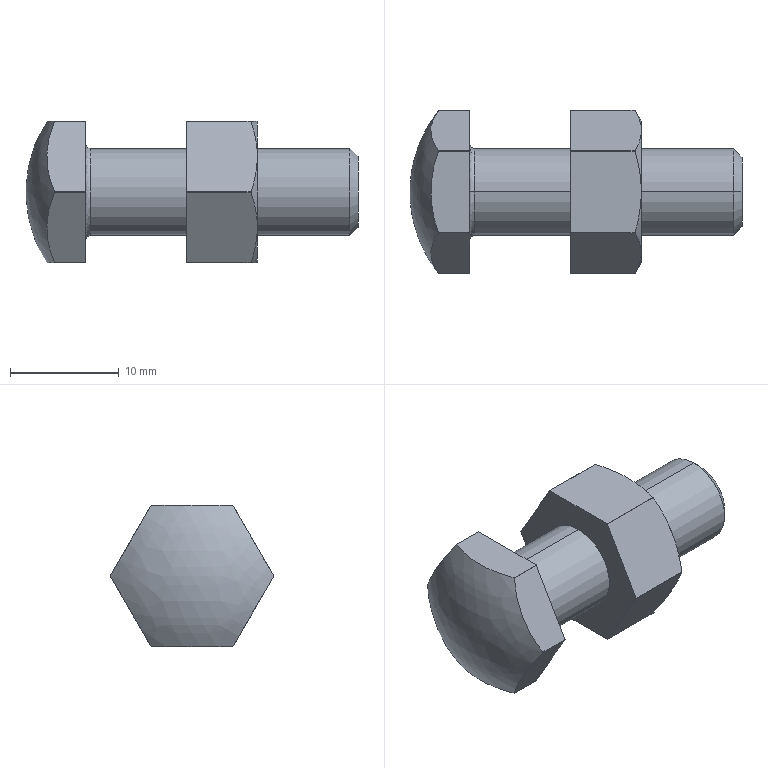Part | STEP file | stbb8_25 | 2 solids | 47 faces | box 30.458 x 15 x 13 mm | volume 2617 mm3 | cylinder 16 | plane 16 | cone 12 | spline 3 | commonest cylinder face diameters 15 x12 6.647 x2 8 x2